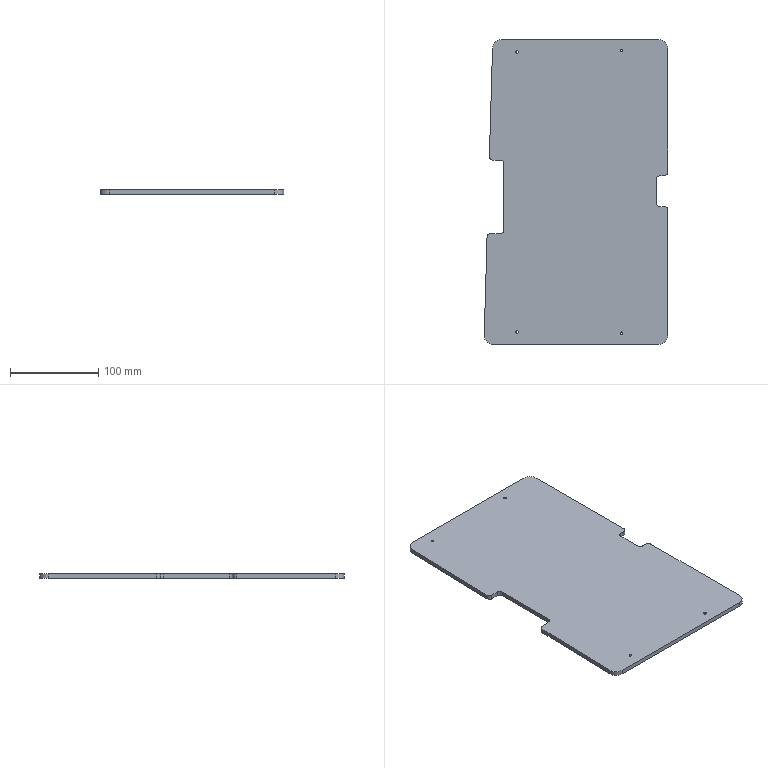Part | NX | features BREP 1 | 1 solid | 30 faces | box 207.864 x 345 x 5 mm | volume 340208 mm3 | cylinder 16 | plane 14 | commonest cylinder face diameters 8 x8 3 x4 20 x4
STEP:
#1=CARTESIAN_POINT('',(52.5,-322.5,0.));
#2=VERTEX_POINT('',#1);
#3=CARTESIAN_POINT('',(52.5,-180.495,0.));
#4=VERTEX_POINT('',#3);
#5=CARTESIAN_POINT('',(52.5,-332.5,0.));
#6=DIRECTION('',(0.,1.,0.));
#7=VECTOR('',#6,1000.);
#8=LINE('',#5,#7);
#9=EDGE_CURVE('',#2,#4,#8,.T.);
#10=ORIENTED_EDGE('',*,*,#9,.T.);
#11=CARTESIAN_POINT('',(52.5,-180.495,5.));
#12=VERTEX_POINT('',#11);
#13=CARTESIAN_POINT('',(52.5,-180.495,5.));
#14=DIRECTION('',(0.,0.,1.));
#15=VECTOR('',#14,1000.);
#16=LINE('',#13,#15);
#17=EDGE_CURVE('',#4,#12,#16,.T.);
#18=ORIENTED_EDGE('',*,*,#17,.T.);
#19=CARTESIAN_POINT('',(52.5,-322.5,5.));
#20=VERTEX_POINT('',#19);
#21=CARTESIAN_POINT('',(52.5,-332.5,5.));
#22=DIRECTION('',(0.,1.,0.));
#23=VECTOR('',#22,1000.);
#24=LINE('',#21,#23);
#25=EDGE_CURVE('',#20,#12,#24,.T.);
#26=ORIENTED_EDGE('',*,*,#25,.F.);
#27=CARTESIAN_POINT('',(52.5,-322.5,5.));
#28=DIRECTION('',(0.,0.,-1.));
#29=VECTOR('',#28,1000.);
#30=LINE('',#27,#29);
#31=EDGE_CURVE('',#20,#2,#30,.T.);
#32=ORIENTED_EDGE('',*,*,#31,.T.);
#33=EDGE_LOOP('',(#10,#18,#26,#32));
#34=FACE_BOUND('',#33,.T.);
#35=CARTESIAN_POINT('',(52.5,-332.5,5.));
#36=DIRECTION('',(-1.,0.,0.));
#37=DIRECTION('',(0.,1.,0.));
#38=AXIS2_PLACEMENT_3D('',#35,#36,#37);
#39=PLANE('',#38);
#40=ADVANCED_FACE('',(#34),#39,.F.);
#41=CARTESIAN_POINT('',(-152.133,-210.884,5.));
#42=VERTEX_POINT('',#41);
#43=CARTESIAN_POINT('',(-155.36,-322.21,5.));
#44=VERTEX_POINT('',#43);
#45=CARTESIAN_POINT('',(-145.658,12.5,5.));
#46=DIRECTION('',(-0.02897,-0.9996,0.));
#47=VECTOR('',#46,1000.);
#48=LINE('',#45,#47);
#49=EDGE_CURVE('',#42,#44,#48,.T.);
#50=ORIENTED_EDGE('',*,*,#49,.F.);
#51=CARTESIAN_POINT('',(-152.133,-210.884,0.));
#52=VERTEX_POINT('',#51);
#53=CARTESIAN_POINT('',(-152.133,-210.884,0.));
#54=DIRECTION('',(0.,0.,-1.));
#55=VECTOR('',#54,1000.);
#56=LINE('',#53,#55);
#57=EDGE_CURVE('',#42,#52,#56,.T.);
#58=ORIENTED_EDGE('',*,*,#57,.T.);
#59=CARTESIAN_POINT('',(-155.36,-322.21,0.));
#60=VERTEX_POINT('',#59);
#61=CARTESIAN_POINT('',(-145.658,12.5,0.));
#62=DIRECTION('',(-0.02897,-0.9996,0.));
#63=VECTOR('',#62,1000.);
#64=LINE('',#61,#63);
#65=EDGE_CURVE('',#52,#60,#64,.T.);
#66=ORIENTED_EDGE('',*,*,#65,.T.);
#67=CARTESIAN_POINT('',(-155.36,-322.21,5.));
#68=DIRECTION('',(0.,0.,1.));
#69=VECTOR('',#68,1000.);
#70=LINE('',#67,#69);
#71=EDGE_CURVE('',#60,#44,#70,.T.);
#72=ORIENTED_EDGE('',*,*,#71,.T.);
#73=EDGE_LOOP('',(#50,#58,#66,#72));
#74=FACE_BOUND('',#73,.T.);
#75=CARTESIAN_POINT('',(-145.658,12.5,5.));
#76=DIRECTION('',(0.9996,-0.02897,0.));
#77=DIRECTION('',(-0.02897,-0.9996,0.));
#78=AXIS2_PLACEMENT_3D('',#75,#76,#77);
#79=PLANE('',#78);
#80=ADVANCED_FACE('',(#74),#79,.F.);
#81=CARTESIAN_POINT('',(-145.94,2.79,0.));
#82=VERTEX_POINT('',#81);
#83=CARTESIAN_POINT('',(-149.495,-119.884,0.));
#84=VERTEX_POINT('',#83);
#85=CARTESIAN_POINT('',(-145.658,12.5,0.));
#86=DIRECTION('',(-0.02897,-0.9996,0.));
#87=VECTOR('',#86,1000.);
#88=LINE('',#85,#87);
#89=EDGE_CURVE('',#82,#84,#88,.T.);
#90=ORIENTED_EDGE('',*,*,#89,.T.);
#91=CARTESIAN_POINT('',(-149.495,-119.884,5.));
#92=VERTEX_POINT('',#91);
#93=CARTESIAN_POINT('',(-149.495,-119.884,5.));
#94=DIRECTION('',(0.,0.,1.));
#95=VECTOR('',#94,1000.);
#96=LINE('',#93,#95);
#97=EDGE_CURVE('',#84,#92,#96,.T.);
#98=ORIENTED_EDGE('',*,*,#97,.T.);
#99=CARTESIAN_POINT('',(-145.94,2.79,5.));
#100=VERTEX_POINT('',#99);
#101=CARTESIAN_POINT('',(-145.658,12.5,5.));
#102=DIRECTION('',(-0.02897,-0.9996,0.));
#103=VECTOR('',#102,1000.);
#104=LINE('',#101,#103);
#105=EDGE_CURVE('',#100,#92,#104,.T.);
#106=ORIENTED_EDGE('',*,*,#105,.F.);
#107=CARTESIAN_POINT('',(-145.94,2.79,5.));
#108=DIRECTION('',(0.,0.,-1.));
#109=VECTOR('',#108,1000.);
#110=LINE('',#107,#109);
#111=EDGE_CURVE('',#100,#82,#110,.T.);
#112=ORIENTED_EDGE('',*,*,#111,.T.);
#113=EDGE_LOOP('',(#90,#98,#106,#112));
#114=FACE_BOUND('',#113,.T.);
#115=CARTESIAN_POINT('',(-145.658,12.5,5.));
#116=DIRECTION('',(0.9996,-0.02897,0.));
#117=DIRECTION('',(-0.02897,-0.9996,0.));
#118=AXIS2_PLACEMENT_3D('',#115,#116,#117);
#119=PLANE('',#118);
#120=ADVANCED_FACE('',(#114),#119,.F.);
#121=CARTESIAN_POINT('',(0.,-318.5,5.));
#122=VERTEX_POINT('',#121);
#123=CARTESIAN_POINT('',(0.,-320.,5.));
#124=DIRECTION('',(0.,0.,-1.));
#125=DIRECTION('',(0.,1.,0.));
#126=AXIS2_PLACEMENT_3D('',#123,#124,#125);
#127=CIRCLE('',#126,1.5);
#128=EDGE_CURVE('',#122,#122,#127,.T.);
#129=ORIENTED_EDGE('',*,*,#128,.T.);
#130=EDGE_LOOP('',(#129));
#131=FACE_BOUND('',#130,.T.);
#132=CARTESIAN_POINT('',(-117.958,-3.,5.));
#133=VERTEX_POINT('',#132);
#134=CARTESIAN_POINT('',(-117.958,-1.5,5.));
#135=DIRECTION('',(0.,0.,1.));
#136=DIRECTION('',(0.,-1.,0.));
#137=AXIS2_PLACEMENT_3D('',#134,#135,#136);
#138=CIRCLE('',#137,1.5);
#139=EDGE_CURVE('',#133,#133,#138,.T.);
#140=ORIENTED_EDGE('',*,*,#139,.F.);
#141=EDGE_LOOP('',(#140));
#142=FACE_BOUND('',#141,.T.);
#143=CARTESIAN_POINT('',(-117.958,-317.,5.));
#144=VERTEX_POINT('',#143);
#145=CARTESIAN_POINT('',(-117.958,-318.5,5.));
#146=DIRECTION('',(0.,0.,-1.));
#147=DIRECTION('',(0.,1.,0.));
#148=AXIS2_PLACEMENT_3D('',#145,#146,#147);
#149=CIRCLE('',#148,1.5);
#150=EDGE_CURVE('',#144,#144,#149,.T.);
#151=ORIENTED_EDGE('',*,*,#150,.T.);
#152=EDGE_LOOP('',(#151));
#153=FACE_BOUND('',#152,.T.);
#154=CARTESIAN_POINT('',(0.,-1.5,5.));
#155=VERTEX_POINT('',#154);
#156=CARTESIAN_POINT('',(0.,0.,5.));
#157=DIRECTION('',(0.,0.,1.));
#158=DIRECTION('',(0.,-1.,0.));
#159=AXIS2_PLACEMENT_3D('',#156,#157,#158);
#160=CIRCLE('',#159,1.5);
#161=EDGE_CURVE('',#155,#155,#160,.T.);
#162=ORIENTED_EDGE('',*,*,#161,.F.);
#163=EDGE_LOOP('',(#162));
#164=FACE_BOUND('',#163,.T.);
#165=CARTESIAN_POINT('',(-148.135,-207.,5.));
#166=VERTEX_POINT('',#165);
#167=CARTESIAN_POINT('',(-137.,-207.,5.));
#168=VERTEX_POINT('',#167);
#169=CARTESIAN_POINT('',(0.,-207.,5.));
#170=DIRECTION('',(1.,0.,0.));
#171=VECTOR('',#170,1000.);
#172=LINE('',#169,#171);
#173=EDGE_CURVE('',#166,#168,#172,.T.);
#174=ORIENTED_EDGE('',*,*,#173,.F.);
#175=CARTESIAN_POINT('',(-148.135,-211.,5.));
#176=DIRECTION('',(0.,0.,1.));
#177=DIRECTION('',(-1.,0.,0.));
#178=AXIS2_PLACEMENT_3D('',#175,#176,#177);
#179=CIRCLE('',#178,4.);
#180=EDGE_CURVE('',#166,#42,#179,.T.);
#181=ORIENTED_EDGE('',*,*,#180,.T.);
#182=ORIENTED_EDGE('',*,*,#49,.T.);
#183=CARTESIAN_POINT('',(-145.364,-332.5,5.));
#184=VERTEX_POINT('',#183);
#185=CARTESIAN_POINT('',(-145.364,-322.5,5.));
#186=DIRECTION('',(0.,0.,1.));
#187=DIRECTION('',(-1.,0.,0.));
#188=AXIS2_PLACEMENT_3D('',#185,#186,#187);
#189=CIRCLE('',#188,10.);
#190=EDGE_CURVE('',#44,#184,#189,.T.);
#191=ORIENTED_EDGE('',*,*,#190,.T.);
#192=CARTESIAN_POINT('',(42.5,-332.5,5.));
#193=VERTEX_POINT('',#192);
#194=CARTESIAN_POINT('',(-155.658,-332.5,5.));
#195=DIRECTION('',(1.,0.,0.));
#196=VECTOR('',#195,1000.);
#197=LINE('',#194,#196);
#198=EDGE_CURVE('',#184,#193,#197,.T.);
#199=ORIENTED_EDGE('',*,*,#198,.T.);
#200=CARTESIAN_POINT('',(42.5,-322.5,5.));
#201=DIRECTION('',(0.,0.,1.));
#202=DIRECTION('',(-1.,0.,0.));
#203=AXIS2_PLACEMENT_3D('',#200,#201,#202);
#204=CIRCLE('',#203,10.);
#205=EDGE_CURVE('',#193,#20,#204,.T.);
#206=ORIENTED_EDGE('',*,*,#205,.T.);
#207=ORIENTED_EDGE('',*,*,#25,.T.);
#208=CARTESIAN_POINT('',(48.5,-176.495,5.));
#209=VERTEX_POINT('',#208);
#210=CARTESIAN_POINT('',(48.5,-180.495,5.));
#211=DIRECTION('',(0.,0.,1.));
#212=DIRECTION('',(-1.,0.,0.));
#213=AXIS2_PLACEMENT_3D('',#210,#211,#212);
#214=CIRCLE('',#213,4.);
#215=EDGE_CURVE('',#12,#209,#214,.T.);
#216=ORIENTED_EDGE('',*,*,#215,.T.);
#217=CARTESIAN_POINT('',(43.5,-176.495,5.));
#218=VERTEX_POINT('',#217);
#219=CARTESIAN_POINT('',(0.,-176.495,5.));
#220=DIRECTION('',(1.,0.,0.));
#221=VECTOR('',#220,1000.);
#222=LINE('',#219,#221);
#223=EDGE_CURVE('',#218,#209,#222,.T.);
#224=ORIENTED_EDGE('',*,*,#223,.F.);
#225=CARTESIAN_POINT('',(39.5,-172.495,5.));
#226=VERTEX_POINT('',#225);
#227=CARTESIAN_POINT('',(43.5,-172.495,5.));
#228=DIRECTION('',(0.,0.,-1.));
#229=DIRECTION('',(-1.,0.,0.));
#230=AXIS2_PLACEMENT_3D('',#227,#228,#229);
#231=CIRCLE('',#230,4.);
#232=EDGE_CURVE('',#218,#226,#231,.T.);
#233=ORIENTED_EDGE('',*,*,#232,.T.);
#234=CARTESIAN_POINT('',(39.5,-145.495,5.));
#235=VERTEX_POINT('',#234);
#236=CARTESIAN_POINT('',(39.5,-320.,5.));
#237=DIRECTION('',(0.,-1.,0.));
#238=VECTOR('',#237,1000.);
#239=LINE('',#236,#238);
#240=EDGE_CURVE('',#235,#226,#239,.T.);
#241=ORIENTED_EDGE('',*,*,#240,.F.);
#242=CARTESIAN_POINT('',(43.5,-141.495,5.));
#243=VERTEX_POINT('',#242);
#244=CARTESIAN_POINT('',(43.5,-145.495,5.));
#245=DIRECTION('',(0.,0.,-1.));
#246=DIRECTION('',(-1.,0.,0.));
#247=AXIS2_PLACEMENT_3D('',#244,#245,#246);
#248=CIRCLE('',#247,4.);
#249=EDGE_CURVE('',#235,#243,#248,.T.);
#250=ORIENTED_EDGE('',*,*,#249,.T.);
#251=CARTESIAN_POINT('',(48.5,-141.495,5.));
#252=VERTEX_POINT('',#251);
#253=CARTESIAN_POINT('',(0.,-141.495,5.));
#254=DIRECTION('',(-1.,0.,0.));
#255=VECTOR('',#254,1000.);
#256=LINE('',#253,#255);
#257=EDGE_CURVE('',#252,#243,#256,.T.);
#258=ORIENTED_EDGE('',*,*,#257,.F.);
#259=CARTESIAN_POINT('',(52.5,-137.495,5.));
#260=VERTEX_POINT('',#259);
#261=CARTESIAN_POINT('',(48.5,-137.495,5.));
#262=DIRECTION('',(0.,0.,1.));
#263=DIRECTION('',(-1.,0.,0.));
#264=AXIS2_PLACEMENT_3D('',#261,#262,#263);
#265=CIRCLE('',#264,4.);
#266=EDGE_CURVE('',#252,#260,#265,.T.);
#267=ORIENTED_EDGE('',*,*,#266,.T.);
#268=CARTESIAN_POINT('',(52.5,2.5,5.));
#269=VERTEX_POINT('',#268);
#270=CARTESIAN_POINT('',(52.5,-332.5,5.));
#271=DIRECTION('',(0.,1.,0.));
#272=VECTOR('',#271,1000.);
#273=LINE('',#270,#272);
#274=EDGE_CURVE('',#260,#269,#273,.T.);
#275=ORIENTED_EDGE('',*,*,#274,.T.);
#276=CARTESIAN_POINT('',(42.5,12.5,5.));
#277=VERTEX_POINT('',#276);
#278=CARTESIAN_POINT('',(42.5,2.5,5.));
#279=DIRECTION('',(0.,0.,1.));
#280=DIRECTION('',(-1.,0.,0.));
#281=AXIS2_PLACEMENT_3D('',#278,#279,#280);
#282=CIRCLE('',#281,10.);
#283=EDGE_CURVE('',#269,#277,#282,.T.);
#284=ORIENTED_EDGE('',*,*,#283,.T.);
#285=CARTESIAN_POINT('',(-135.944,12.5,5.));
#286=VERTEX_POINT('',#285);
#287=CARTESIAN_POINT('',(52.5,12.5,5.));
#288=DIRECTION('',(-1.,0.,0.));
#289=VECTOR('',#288,1000.);
#290=LINE('',#287,#289);
#291=EDGE_CURVE('',#277,#286,#290,.T.);
#292=ORIENTED_EDGE('',*,*,#291,.T.);
#293=CARTESIAN_POINT('',(-135.944,2.5,5.));
#294=DIRECTION('',(0.,0.,1.));
#295=DIRECTION('',(-1.,0.,0.));
#296=AXIS2_PLACEMENT_3D('',#293,#294,#295);
#297=CIRCLE('',#296,10.);
#298=EDGE_CURVE('',#286,#100,#297,.T.);
#299=ORIENTED_EDGE('',*,*,#298,.T.);
#300=ORIENTED_EDGE('',*,*,#105,.T.);
#301=CARTESIAN_POINT('',(-145.497,-124.,5.));
#302=VERTEX_POINT('',#301);
#303=CARTESIAN_POINT('',(-145.497,-120.,5.));
#304=DIRECTION('',(0.,0.,1.));
#305=DIRECTION('',(-1.,0.,0.));
#306=AXIS2_PLACEMENT_3D('',#303,#304,#305);
#307=CIRCLE('',#306,4.);
#308=EDGE_CURVE('',#92,#302,#307,.T.);
#309=ORIENTED_EDGE('',*,*,#308,.T.);
#310=CARTESIAN_POINT('',(-137.,-124.,5.));
#311=VERTEX_POINT('',#310);
#312=CARTESIAN_POINT('',(0.,-124.,5.));
#313=DIRECTION('',(-1.,0.,0.));
#314=VECTOR('',#313,1000.);
#315=LINE('',#312,#314);
#316=EDGE_CURVE('',#311,#302,#315,.T.);
#317=ORIENTED_EDGE('',*,*,#316,.F.);
#318=CARTESIAN_POINT('',(-133.,-128.,5.));
#319=VERTEX_POINT('',#318);
#320=CARTESIAN_POINT('',(-137.,-128.,5.));
#321=DIRECTION('',(0.,0.,-1.));
#322=DIRECTION('',(-1.,0.,0.));
#323=AXIS2_PLACEMENT_3D('',#320,#321,#322);
#324=CIRCLE('',#323,4.);
#325=EDGE_CURVE('',#311,#319,#324,.T.);
#326=ORIENTED_EDGE('',*,*,#325,.T.);
#327=CARTESIAN_POINT('',(-133.,-203.,5.));
#328=VERTEX_POINT('',#327);
#329=CARTESIAN_POINT('',(-133.,-320.,5.));
#330=DIRECTION('',(0.,1.,0.));
#331=VECTOR('',#330,1000.);
#332=LINE('',#329,#331);
#333=EDGE_CURVE('',#328,#319,#332,.T.);
#334=ORIENTED_EDGE('',*,*,#333,.F.);
#335=CARTESIAN_POINT('',(-137.,-203.,5.));
#336=DIRECTION('',(0.,0.,-1.));
#337=DIRECTION('',(-1.,0.,0.));
#338=AXIS2_PLACEMENT_3D('',#335,#336,#337);
#339=CIRCLE('',#338,4.);
#340=EDGE_CURVE('',#328,#168,#339,.T.);
#341=ORIENTED_EDGE('',*,*,#340,.T.);
#342=EDGE_LOOP('',(#174,#181,#182,#191,#199,#206,#207,#216,#224,#233,#241,#250,#258,#267,#275,#284,#292,#299,#300,#309,#317,#326,#334,#341));
#343=FACE_BOUND('',#342,.T.);
#344=CARTESIAN_POINT('',(0.,-320.,5.));
#345=DIRECTION('',(0.,0.,-1.));
#346=DIRECTION('',(1.,0.,0.));
#347=AXIS2_PLACEMENT_3D('',#344,#345,#346);
#348=PLANE('',#347);
#349=ADVANCED_FACE('',(#131,#142,#153,#164,#343),#348,.F.);
#350=CARTESIAN_POINT('',(0.,-318.5,0.));
#351=VERTEX_POINT('',#350);
#352=CARTESIAN_POINT('',(0.,-320.,0.));
#353=DIRECTION('',(0.,0.,-1.));
#354=DIRECTION('',(0.,1.,0.));
#355=AXIS2_PLACEMENT_3D('',#352,#353,#354);
#356=CIRCLE('',#355,1.5);
#357=EDGE_CURVE('',#351,#351,#356,.T.);
#358=ORIENTED_EDGE('',*,*,#357,.F.);
#359=EDGE_LOOP('',(#358));
#360=FACE_BOUND('',#359,.T.);
#361=CARTESIAN_POINT('',(-117.958,-3.,0.));
#362=VERTEX_POINT('',#361);
#363=CARTESIAN_POINT('',(-117.958,-1.5,0.));
#364=DIRECTION('',(0.,0.,1.));
#365=DIRECTION('',(0.,-1.,0.));
#366=AXIS2_PLACEMENT_3D('',#363,#364,#365);
#367=CIRCLE('',#366,1.5);
#368=EDGE_CURVE('',#362,#362,#367,.T.);
#369=ORIENTED_EDGE('',*,*,#368,.T.);
#370=EDGE_LOOP('',(#369));
#371=FACE_BOUND('',#370,.T.);
#372=CARTESIAN_POINT('',(-117.958,-317.,0.));
#373=VERTEX_POINT('',#372);
#374=CARTESIAN_POINT('',(-117.958,-318.5,0.));
#375=DIRECTION('',(0.,0.,-1.));
#376=DIRECTION('',(0.,1.,0.));
#377=AXIS2_PLACEMENT_3D('',#374,#375,#376);
#378=CIRCLE('',#377,1.5);
#379=EDGE_CURVE('',#373,#373,#378,.T.);
#380=ORIENTED_EDGE('',*,*,#379,.F.);
#381=EDGE_LOOP('',(#380));
#382=FACE_BOUND('',#381,.T.);
#383=CARTESIAN_POINT('',(0.,-1.5,0.));
#384=VERTEX_POINT('',#383);
#385=CARTESIAN_POINT('',(0.,0.,0.));
#386=DIRECTION('',(0.,0.,1.));
#387=DIRECTION('',(0.,-1.,0.));
#388=AXIS2_PLACEMENT_3D('',#385,#386,#387);
#389=CIRCLE('',#388,1.5);
#390=EDGE_CURVE('',#384,#384,#389,.T.);
#391=ORIENTED_EDGE('',*,*,#390,.T.);
#392=EDGE_LOOP('',(#391));
#393=FACE_BOUND('',#392,.T.);
#394=ORIENTED_EDGE('',*,*,#65,.F.);
#395=CARTESIAN_POINT('',(-148.135,-207.,0.));
#396=VERTEX_POINT('',#395);
#397=CARTESIAN_POINT('',(-148.135,-211.,0.));
#398=DIRECTION('',(0.,0.,-1.));
#399=DIRECTION('',(-1.,0.,0.));
#400=AXIS2_PLACEMENT_3D('',#397,#398,#399);
#401=CIRCLE('',#400,4.);
#402=EDGE_CURVE('',#52,#396,#401,.T.);
#403=ORIENTED_EDGE('',*,*,#402,.T.);
#404=CARTESIAN_POINT('',(-137.,-207.,0.));
#405=VERTEX_POINT('',#404);
#406=CARTESIAN_POINT('',(0.,-207.,0.));
#407=DIRECTION('',(1.,0.,0.));
#408=VECTOR('',#407,1000.);
#409=LINE('',#406,#408);
#410=EDGE_CURVE('',#396,#405,#409,.T.);
#411=ORIENTED_EDGE('',*,*,#410,.T.);
#412=CARTESIAN_POINT('',(-133.,-203.,0.));
#413=VERTEX_POINT('',#412);
#414=CARTESIAN_POINT('',(-137.,-203.,0.));
#415=DIRECTION('',(0.,0.,1.));
#416=DIRECTION('',(-1.,0.,0.));
#417=AXIS2_PLACEMENT_3D('',#414,#415,#416);
#418=CIRCLE('',#417,4.);
#419=EDGE_CURVE('',#405,#413,#418,.T.);
#420=ORIENTED_EDGE('',*,*,#419,.T.);
#421=CARTESIAN_POINT('',(-133.,-128.,0.));
#422=VERTEX_POINT('',#421);
#423=CARTESIAN_POINT('',(-133.,-320.,0.));
#424=DIRECTION('',(0.,1.,0.));
#425=VECTOR('',#424,1000.);
#426=LINE('',#423,#425);
#427=EDGE_CURVE('',#413,#422,#426,.T.);
#428=ORIENTED_EDGE('',*,*,#427,.T.);
#429=CARTESIAN_POINT('',(-137.,-124.,0.));
#430=VERTEX_POINT('',#429);
#431=CARTESIAN_POINT('',(-137.,-128.,0.));
#432=DIRECTION('',(0.,0.,1.));
#433=DIRECTION('',(-1.,0.,0.));
#434=AXIS2_PLACEMENT_3D('',#431,#432,#433);
#435=CIRCLE('',#434,4.);
#436=EDGE_CURVE('',#422,#430,#435,.T.);
#437=ORIENTED_EDGE('',*,*,#436,.T.);
#438=CARTESIAN_POINT('',(-145.497,-124.,0.));
#439=VERTEX_POINT('',#438);
#440=CARTESIAN_POINT('',(0.,-124.,0.));
#441=DIRECTION('',(-1.,0.,0.));
#442=VECTOR('',#441,1000.);
#443=LINE('',#440,#442);
#444=EDGE_CURVE('',#430,#439,#443,.T.);
#445=ORIENTED_EDGE('',*,*,#444,.T.);
#446=CARTESIAN_POINT('',(-145.497,-120.,0.));
#447=DIRECTION('',(0.,0.,-1.));
#448=DIRECTION('',(-1.,0.,0.));
#449=AXIS2_PLACEMENT_3D('',#446,#447,#448);
#450=CIRCLE('',#449,4.);
#451=EDGE_CURVE('',#439,#84,#450,.T.);
#452=ORIENTED_EDGE('',*,*,#451,.T.);
#453=ORIENTED_EDGE('',*,*,#89,.F.);
#454=CARTESIAN_POINT('',(-135.944,12.5,0.));
#455=VERTEX_POINT('',#454);
#456=CARTESIAN_POINT('',(-135.944,2.5,0.));
#457=DIRECTION('',(0.,0.,-1.));
#458=DIRECTION('',(-1.,0.,0.));
#459=AXIS2_PLACEMENT_3D('',#456,#457,#458);
#460=CIRCLE('',#459,10.);
#461=EDGE_CURVE('',#82,#455,#460,.T.);
#462=ORIENTED_EDGE('',*,*,#461,.T.);
#463=CARTESIAN_POINT('',(42.5,12.5,0.));
#464=VERTEX_POINT('',#463);
#465=CARTESIAN_POINT('',(52.5,12.5,0.));
#466=DIRECTION('',(-1.,0.,0.));
#467=VECTOR('',#466,1000.);
#468=LINE('',#465,#467);
#469=EDGE_CURVE('',#464,#455,#468,.T.);
#470=ORIENTED_EDGE('',*,*,#469,.F.);
#471=CARTESIAN_POINT('',(52.5,2.5,0.));
#472=VERTEX_POINT('',#471);
#473=CARTESIAN_POINT('',(42.5,2.5,0.));
#474=DIRECTION('',(0.,0.,-1.));
#475=DIRECTION('',(-1.,0.,0.));
#476=AXIS2_PLACEMENT_3D('',#473,#474,#475);
#477=CIRCLE('',#476,10.);
#478=EDGE_CURVE('',#464,#472,#477,.T.);
#479=ORIENTED_EDGE('',*,*,#478,.T.);
#480=CARTESIAN_POINT('',(52.5,-137.495,0.));
#481=VERTEX_POINT('',#480);
#482=CARTESIAN_POINT('',(52.5,-332.5,0.));
#483=DIRECTION('',(0.,1.,0.));
#484=VECTOR('',#483,1000.);
#485=LINE('',#482,#484);
#486=EDGE_CURVE('',#481,#472,#485,.T.);
#487=ORIENTED_EDGE('',*,*,#486,.F.);
#488=CARTESIAN_POINT('',(48.5,-141.495,0.));
#489=VERTEX_POINT('',#488);
#490=CARTESIAN_POINT('',(48.5,-137.495,0.));
#491=DIRECTION('',(0.,0.,-1.));
#492=DIRECTION('',(-1.,0.,0.));
#493=AXIS2_PLACEMENT_3D('',#490,#491,#492);
#494=CIRCLE('',#493,4.);
#495=EDGE_CURVE('',#481,#489,#494,.T.);
#496=ORIENTED_EDGE('',*,*,#495,.T.);
#497=CARTESIAN_POINT('',(43.5,-141.495,0.));
#498=VERTEX_POINT('',#497);
#499=CARTESIAN_POINT('',(0.,-141.495,0.));
#500=DIRECTION('',(-1.,0.,0.));
#501=VECTOR('',#500,1000.);
#502=LINE('',#499,#501);
#503=EDGE_CURVE('',#489,#498,#502,.T.);
#504=ORIENTED_EDGE('',*,*,#503,.T.);
#505=CARTESIAN_POINT('',(39.5,-145.495,0.));
#506=VERTEX_POINT('',#505);
#507=CARTESIAN_POINT('',(43.5,-145.495,0.));
#508=DIRECTION('',(0.,0.,1.));
#509=DIRECTION('',(-1.,0.,0.));
#510=AXIS2_PLACEMENT_3D('',#507,#508,#509);
#511=CIRCLE('',#510,4.);
#512=EDGE_CURVE('',#498,#506,#511,.T.);
#513=ORIENTED_EDGE('',*,*,#512,.T.);
#514=CARTESIAN_POINT('',(39.5,-172.495,0.));
#515=VERTEX_POINT('',#514);
#516=CARTESIAN_POINT('',(39.5,-320.,0.));
#517=DIRECTION('',(0.,-1.,0.));
#518=VECTOR('',#517,1000.);
#519=LINE('',#516,#518);
#520=EDGE_CURVE('',#506,#515,#519,.T.);
#521=ORIENTED_EDGE('',*,*,#520,.T.);
#522=CARTESIAN_POINT('',(43.5,-176.495,0.));
#523=VERTEX_POINT('',#522);
#524=CARTESIAN_POINT('',(43.5,-172.495,0.));
#525=DIRECTION('',(0.,0.,1.));
#526=DIRECTION('',(-1.,0.,0.));
#527=AXIS2_PLACEMENT_3D('',#524,#525,#526);
#528=CIRCLE('',#527,4.);
#529=EDGE_CURVE('',#515,#523,#528,.T.);
#530=ORIENTED_EDGE('',*,*,#529,.T.);
#531=CARTESIAN_POINT('',(48.5,-176.495,0.));
#532=VERTEX_POINT('',#531);
#533=CARTESIAN_POINT('',(0.,-176.495,0.));
#534=DIRECTION('',(1.,0.,0.));
#535=VECTOR('',#534,1000.);
#536=LINE('',#533,#535);
#537=EDGE_CURVE('',#523,#532,#536,.T.);
#538=ORIENTED_EDGE('',*,*,#537,.T.);
#539=CARTESIAN_POINT('',(48.5,-180.495,0.));
#540=DIRECTION('',(0.,0.,-1.));
#541=DIRECTION('',(-1.,0.,0.));
#542=AXIS2_PLACEMENT_3D('',#539,#540,#541);
#543=CIRCLE('',#542,4.);
#544=EDGE_CURVE('',#532,#4,#543,.T.);
#545=ORIENTED_EDGE('',*,*,#544,.T.);
#546=ORIENTED_EDGE('',*,*,#9,.F.);
#547=CARTESIAN_POINT('',(42.5,-332.5,0.));
#548=VERTEX_POINT('',#547);
#549=CARTESIAN_POINT('',(42.5,-322.5,0.));
#550=DIRECTION('',(0.,0.,-1.));
#551=DIRECTION('',(-1.,0.,0.));
#552=AXIS2_PLACEMENT_3D('',#549,#550,#551);
#553=CIRCLE('',#552,10.);
#554=EDGE_CURVE('',#2,#548,#553,.T.);
#555=ORIENTED_EDGE('',*,*,#554,.T.);
#556=CARTESIAN_POINT('',(-145.364,-332.5,0.));
#557=VERTEX_POINT('',#556);
#558=CARTESIAN_POINT('',(-155.658,-332.5,0.));
#559=DIRECTION('',(1.,0.,0.));
#560=VECTOR('',#559,1000.);
#561=LINE('',#558,#560);
#562=EDGE_CURVE('',#557,#548,#561,.T.);
#563=ORIENTED_EDGE('',*,*,#562,.F.);
#564=CARTESIAN_POINT('',(-145.364,-322.5,0.));
#565=DIRECTION('',(0.,0.,-1.));
#566=DIRECTION('',(-1.,0.,0.));
#567=AXIS2_PLACEMENT_3D('',#564,#565,#566);
#568=CIRCLE('',#567,10.);
#569=EDGE_CURVE('',#557,#60,#568,.T.);
#570=ORIENTED_EDGE('',*,*,#569,.T.);
#571=EDGE_LOOP('',(#394,#403,#411,#420,#428,#437,#445,#452,#453,#462,#470,#479,#487,#496,#504,#513,#521,#530,#538,#545,#546,#555,#563,#570));
#572=FACE_BOUND('',#571,.T.);
#573=CARTESIAN_POINT('',(0.,-320.,0.));
#574=DIRECTION('',(0.,0.,-1.));
#575=DIRECTION('',(1.,0.,0.));
#576=AXIS2_PLACEMENT_3D('',#573,#574,#575);
#577=PLANE('',#576);
#578=ADVANCED_FACE('',(#360,#371,#382,#393,#572),#577,.T.);
#579=ORIENTED_EDGE('',*,*,#198,.F.);
#580=CARTESIAN_POINT('',(-145.364,-332.5,5.));
#581=DIRECTION('',(0.,0.,-1.));
#582=VECTOR('',#581,1000.);
#583=LINE('',#580,#582);
#584=EDGE_CURVE('',#184,#557,#583,.T.);
#585=ORIENTED_EDGE('',*,*,#584,.T.);
#586=ORIENTED_EDGE('',*,*,#562,.T.);
#587=CARTESIAN_POINT('',(42.5,-332.5,5.));
#588=DIRECTION('',(0.,0.,1.));
#589=VECTOR('',#588,1000.);
#590=LINE('',#587,#589);
#591=EDGE_CURVE('',#548,#193,#590,.T.);
#592=ORIENTED_EDGE('',*,*,#591,.T.);
#593=EDGE_LOOP('',(#579,#585,#586,#592));
#594=FACE_BOUND('',#593,.T.);
#595=CARTESIAN_POINT('',(-155.658,-332.5,5.));
#596=DIRECTION('',(0.,1.,0.));
#597=DIRECTION('',(1.,0.,0.));
#598=AXIS2_PLACEMENT_3D('',#595,#596,#597);
#599=PLANE('',#598);
#600=ADVANCED_FACE('',(#594),#599,.F.);
#601=ORIENTED_EDGE('',*,*,#274,.F.);
#602=CARTESIAN_POINT('',(52.5,-137.495,0.));
#603=DIRECTION('',(0.,0.,-1.));
#604=VECTOR('',#603,1000.);
#605=LINE('',#602,#604);
#606=EDGE_CURVE('',#260,#481,#605,.T.);
#607=ORIENTED_EDGE('',*,*,#606,.T.);
#608=ORIENTED_EDGE('',*,*,#486,.T.);
#609=CARTESIAN_POINT('',(52.5,2.5,5.));
#610=DIRECTION('',(0.,0.,1.));
#611=VECTOR('',#610,1000.);
#612=LINE('',#609,#611);
#613=EDGE_CURVE('',#472,#269,#612,.T.);
#614=ORIENTED_EDGE('',*,*,#613,.T.);
#615=EDGE_LOOP('',(#601,#607,#608,#614));
#616=FACE_BOUND('',#615,.T.);
#617=CARTESIAN_POINT('',(52.5,-332.5,5.));
#618=DIRECTION('',(-1.,0.,0.));
#619=DIRECTION('',(0.,1.,0.));
#620=AXIS2_PLACEMENT_3D('',#617,#618,#619);
#621=PLANE('',#620);
#622=ADVANCED_FACE('',(#616),#621,.F.);
#623=ORIENTED_EDGE('',*,*,#150,.F.);
#624=EDGE_LOOP('',(#623));
#625=FACE_BOUND('',#624,.T.);
#626=ORIENTED_EDGE('',*,*,#379,.T.);
#627=EDGE_LOOP('',(#626));
#628=FACE_BOUND('',#627,.T.);
#629=CARTESIAN_POINT('',(-117.958,-318.5,5.));
#630=DIRECTION('',(0.,0.,-1.));
#631=DIRECTION('',(1.,0.,0.));
#632=AXIS2_PLACEMENT_3D('',#629,#630,#631);
#633=CYLINDRICAL_SURFACE('',#632,1.5);
#634=ADVANCED_FACE('',(#625,#628),#633,.F.);
#635=ORIENTED_EDGE('',*,*,#139,.T.);
#636=EDGE_LOOP('',(#635));
#637=FACE_BOUND('',#636,.T.);
#638=ORIENTED_EDGE('',*,*,#368,.F.);
#639=EDGE_LOOP('',(#638));
#640=FACE_BOUND('',#639,.T.);
#641=CARTESIAN_POINT('',(-117.958,-1.5,5.));
#642=DIRECTION('',(0.,0.,-1.));
#643=DIRECTION('',(1.,0.,0.));
#644=AXIS2_PLACEMENT_3D('',#641,#642,#643);
#645=CYLINDRICAL_SURFACE('',#644,1.5);
#646=ADVANCED_FACE('',(#637,#640),#645,.F.);
#647=ORIENTED_EDGE('',*,*,#128,.F.);
#648=EDGE_LOOP('',(#647));
#649=FACE_BOUND('',#648,.T.);
#650=ORIENTED_EDGE('',*,*,#357,.T.);
#651=EDGE_LOOP('',(#650));
#652=FACE_BOUND('',#651,.T.);
#653=CARTESIAN_POINT('',(0.,-320.,5.));
#654=DIRECTION('',(0.,0.,-1.));
#655=DIRECTION('',(1.,0.,0.));
#656=AXIS2_PLACEMENT_3D('',#653,#654,#655);
#657=CYLINDRICAL_SURFACE('',#656,1.5);
#658=ADVANCED_FACE('',(#649,#652),#657,.F.);
#659=ORIENTED_EDGE('',*,*,#469,.T.);
#660=CARTESIAN_POINT('',(-135.944,12.5,5.));
#661=DIRECTION('',(0.,0.,1.));
#662=VECTOR('',#661,1000.);
#663=LINE('',#660,#662);
#664=EDGE_CURVE('',#455,#286,#663,.T.);
#665=ORIENTED_EDGE('',*,*,#664,.T.);
#666=ORIENTED_EDGE('',*,*,#291,.F.);
#667=CARTESIAN_POINT('',(42.5,12.5,5.));
#668=DIRECTION('',(0.,0.,-1.));
#669=VECTOR('',#668,1000.);
#670=LINE('',#667,#669);
#671=EDGE_CURVE('',#277,#464,#670,.T.);
#672=ORIENTED_EDGE('',*,*,#671,.T.);
#673=EDGE_LOOP('',(#659,#665,#666,#672));
#674=FACE_BOUND('',#673,.T.);
#675=CARTESIAN_POINT('',(52.5,12.5,5.));
#676=DIRECTION('',(0.,-1.,0.));
#677=DIRECTION('',(0.,0.,1.));
#678=AXIS2_PLACEMENT_3D('',#675,#676,#677);
#679=PLANE('',#678);
#680=ADVANCED_FACE('',(#674),#679,.F.);
#681=ORIENTED_EDGE('',*,*,#161,.T.);
#682=EDGE_LOOP('',(#681));
#683=FACE_BOUND('',#682,.T.);
#684=ORIENTED_EDGE('',*,*,#390,.F.);
#685=EDGE_LOOP('',(#684));
#686=FACE_BOUND('',#685,.T.);
#687=CARTESIAN_POINT('',(0.,0.,5.));
#688=DIRECTION('',(0.,0.,-1.));
#689=DIRECTION('',(1.,0.,0.));
#690=AXIS2_PLACEMENT_3D('',#687,#688,#689);
#691=CYLINDRICAL_SURFACE('',#690,1.5);
#692=ADVANCED_FACE('',(#683,#686),#691,.F.);
#693=ORIENTED_EDGE('',*,*,#190,.F.);
#694=ORIENTED_EDGE('',*,*,#71,.F.);
#695=ORIENTED_EDGE('',*,*,#569,.F.);
#696=ORIENTED_EDGE('',*,*,#584,.F.);
#697=EDGE_LOOP('',(#693,#694,#695,#696));
#698=FACE_BOUND('',#697,.T.);
#699=CARTESIAN_POINT('',(-145.364,-322.5,5.));
#700=DIRECTION('',(0.,0.,-1.));
#701=DIRECTION('',(1.,0.,0.));
#702=AXIS2_PLACEMENT_3D('',#699,#700,#701);
#703=CYLINDRICAL_SURFACE('',#702,10.);
#704=ADVANCED_FACE('',(#698),#703,.T.);
#705=ORIENTED_EDGE('',*,*,#298,.F.);
#706=ORIENTED_EDGE('',*,*,#664,.F.);
#707=ORIENTED_EDGE('',*,*,#461,.F.);
#708=ORIENTED_EDGE('',*,*,#111,.F.);
#709=EDGE_LOOP('',(#705,#706,#707,#708));
#710=FACE_BOUND('',#709,.T.);
#711=CARTESIAN_POINT('',(-135.944,2.5,5.));
#712=DIRECTION('',(0.,0.,-1.));
#713=DIRECTION('',(1.,0.,0.));
#714=AXIS2_PLACEMENT_3D('',#711,#712,#713);
#715=CYLINDRICAL_SURFACE('',#714,10.);
#716=ADVANCED_FACE('',(#710),#715,.T.);
#717=ORIENTED_EDGE('',*,*,#283,.F.);
#718=ORIENTED_EDGE('',*,*,#613,.F.);
#719=ORIENTED_EDGE('',*,*,#478,.F.);
#720=ORIENTED_EDGE('',*,*,#671,.F.);
#721=EDGE_LOOP('',(#717,#718,#719,#720));
#722=FACE_BOUND('',#721,.T.);
#723=CARTESIAN_POINT('',(42.5,2.5,5.));
#724=DIRECTION('',(0.,0.,-1.));
#725=DIRECTION('',(1.,0.,0.));
#726=AXIS2_PLACEMENT_3D('',#723,#724,#725);
#727=CYLINDRICAL_SURFACE('',#726,10.);
#728=ADVANCED_FACE('',(#722),#727,.T.);
#729=ORIENTED_EDGE('',*,*,#205,.F.);
#730=ORIENTED_EDGE('',*,*,#591,.F.);
#731=ORIENTED_EDGE('',*,*,#554,.F.);
#732=ORIENTED_EDGE('',*,*,#31,.F.);
#733=EDGE_LOOP('',(#729,#730,#731,#732));
#734=FACE_BOUND('',#733,.T.);
#735=CARTESIAN_POINT('',(42.5,-322.5,5.));
#736=DIRECTION('',(0.,0.,-1.));
#737=DIRECTION('',(1.,0.,0.));
#738=AXIS2_PLACEMENT_3D('',#735,#736,#737);
#739=CYLINDRICAL_SURFACE('',#738,10.);
#740=ADVANCED_FACE('',(#734),#739,.T.);
#741=ORIENTED_EDGE('',*,*,#410,.F.);
#742=CARTESIAN_POINT('',(-148.135,-207.,5.));
#743=DIRECTION('',(0.,0.,1.));
#744=VECTOR('',#743,1000.);
#745=LINE('',#742,#744);
#746=EDGE_CURVE('',#396,#166,#745,.T.);
#747=ORIENTED_EDGE('',*,*,#746,.T.);
#748=ORIENTED_EDGE('',*,*,#173,.T.);
#749=CARTESIAN_POINT('',(-137.,-207.,0.));
#750=DIRECTION('',(0.,0.,-1.));
#751=VECTOR('',#750,1000.);
#752=LINE('',#749,#751);
#753=EDGE_CURVE('',#168,#405,#752,.T.);
#754=ORIENTED_EDGE('',*,*,#753,.T.);
#755=EDGE_LOOP('',(#741,#747,#748,#754));
#756=FACE_BOUND('',#755,.T.);
#757=CARTESIAN_POINT('',(-158.,-207.,25.));
#758=DIRECTION('',(0.,1.,0.));
#759=DIRECTION('',(1.,0.,0.));
#760=AXIS2_PLACEMENT_3D('',#757,#758,#759);
#761=PLANE('',#760);
#762=ADVANCED_FACE('',(#756),#761,.T.);
#763=ORIENTED_EDGE('',*,*,#427,.F.);
#764=CARTESIAN_POINT('',(-133.,-203.,5.));
#765=DIRECTION('',(0.,0.,1.));
#766=VECTOR('',#765,1000.);
#767=LINE('',#764,#766);
#768=EDGE_CURVE('',#413,#328,#767,.T.);
#769=ORIENTED_EDGE('',*,*,#768,.T.);
#770=ORIENTED_EDGE('',*,*,#333,.T.);
#771=CARTESIAN_POINT('',(-133.,-128.,0.));
#772=DIRECTION('',(0.,0.,-1.));
#773=VECTOR('',#772,1000.);
#774=LINE('',#771,#773);
#775=EDGE_CURVE('',#319,#422,#774,.T.);
#776=ORIENTED_EDGE('',*,*,#775,.T.);
#777=EDGE_LOOP('',(#763,#769,#770,#776));
#778=FACE_BOUND('',#777,.T.);
#779=CARTESIAN_POINT('',(-133.,-207.,25.));
#780=DIRECTION('',(-1.,0.,0.));
#781=DIRECTION('',(0.,1.,0.));
#782=AXIS2_PLACEMENT_3D('',#779,#780,#781);
#783=PLANE('',#782);
#784=ADVANCED_FACE('',(#778),#783,.T.);
#785=ORIENTED_EDGE('',*,*,#444,.F.);
#786=CARTESIAN_POINT('',(-137.,-124.,5.));
#787=DIRECTION('',(0.,0.,1.));
#788=VECTOR('',#787,1000.);
#789=LINE('',#786,#788);
#790=EDGE_CURVE('',#430,#311,#789,.T.);
#791=ORIENTED_EDGE('',*,*,#790,.T.);
#792=ORIENTED_EDGE('',*,*,#316,.T.);
#793=CARTESIAN_POINT('',(-145.497,-124.,0.));
#794=DIRECTION('',(0.,0.,-1.));
#795=VECTOR('',#794,1000.);
#796=LINE('',#793,#795);
#797=EDGE_CURVE('',#302,#439,#796,.T.);
#798=ORIENTED_EDGE('',*,*,#797,.T.);
#799=EDGE_LOOP('',(#785,#791,#792,#798));
#800=FACE_BOUND('',#799,.T.);
#801=CARTESIAN_POINT('',(-133.,-124.,25.));
#802=DIRECTION('',(0.,-1.,0.));
#803=DIRECTION('',(-1.,0.,0.));
#804=AXIS2_PLACEMENT_3D('',#801,#802,#803);
#805=PLANE('',#804);
#806=ADVANCED_FACE('',(#800),#805,.T.);
#807=ORIENTED_EDGE('',*,*,#240,.T.);
#808=CARTESIAN_POINT('',(39.5,-172.495,0.));
#809=DIRECTION('',(0.,0.,-1.));
#810=VECTOR('',#809,1000.);
#811=LINE('',#808,#810);
#812=EDGE_CURVE('',#226,#515,#811,.T.);
#813=ORIENTED_EDGE('',*,*,#812,.T.);
#814=ORIENTED_EDGE('',*,*,#520,.F.);
#815=CARTESIAN_POINT('',(39.5,-145.495,5.));
#816=DIRECTION('',(0.,0.,1.));
#817=VECTOR('',#816,1000.);
#818=LINE('',#815,#817);
#819=EDGE_CURVE('',#506,#235,#818,.T.);
#820=ORIENTED_EDGE('',*,*,#819,.T.);
#821=EDGE_LOOP('',(#807,#813,#814,#820));
#822=FACE_BOUND('',#821,.T.);
#823=CARTESIAN_POINT('',(39.5,-141.495,25.));
#824=DIRECTION('',(1.,0.,0.));
#825=DIRECTION('',(0.,-1.,0.));
#826=AXIS2_PLACEMENT_3D('',#823,#824,#825);
#827=PLANE('',#826);
#828=ADVANCED_FACE('',(#822),#827,.T.);
#829=ORIENTED_EDGE('',*,*,#223,.T.);
#830=CARTESIAN_POINT('',(48.5,-176.495,0.));
#831=DIRECTION('',(0.,0.,-1.));
#832=VECTOR('',#831,1000.);
#833=LINE('',#830,#832);
#834=EDGE_CURVE('',#209,#532,#833,.T.);
#835=ORIENTED_EDGE('',*,*,#834,.T.);
#836=ORIENTED_EDGE('',*,*,#537,.F.);
#837=CARTESIAN_POINT('',(43.5,-176.495,5.));
#838=DIRECTION('',(0.,0.,1.));
#839=VECTOR('',#838,1000.);
#840=LINE('',#837,#839);
#841=EDGE_CURVE('',#523,#218,#840,.T.);
#842=ORIENTED_EDGE('',*,*,#841,.T.);
#843=EDGE_LOOP('',(#829,#835,#836,#842));
#844=FACE_BOUND('',#843,.T.);
#845=CARTESIAN_POINT('',(39.5,-176.495,25.));
#846=DIRECTION('',(0.,1.,0.));
#847=DIRECTION('',(1.,0.,0.));
#848=AXIS2_PLACEMENT_3D('',#845,#846,#847);
#849=PLANE('',#848);
#850=ADVANCED_FACE('',(#844),#849,.T.);
#851=ORIENTED_EDGE('',*,*,#503,.F.);
#852=CARTESIAN_POINT('',(48.5,-141.495,5.));
#853=DIRECTION('',(0.,0.,1.));
#854=VECTOR('',#853,1000.);
#855=LINE('',#852,#854);
#856=EDGE_CURVE('',#489,#252,#855,.T.);
#857=ORIENTED_EDGE('',*,*,#856,.T.);
#858=ORIENTED_EDGE('',*,*,#257,.T.);
#859=CARTESIAN_POINT('',(43.5,-141.495,0.));
#860=DIRECTION('',(0.,0.,-1.));
#861=VECTOR('',#860,1000.);
#862=LINE('',#859,#861);
#863=EDGE_CURVE('',#243,#498,#862,.T.);
#864=ORIENTED_EDGE('',*,*,#863,.T.);
#865=EDGE_LOOP('',(#851,#857,#858,#864));
#866=FACE_BOUND('',#865,.T.);
#867=CARTESIAN_POINT('',(52.5,-141.495,25.));
#868=DIRECTION('',(0.,-1.,0.));
#869=DIRECTION('',(-1.,0.,0.));
#870=AXIS2_PLACEMENT_3D('',#867,#868,#869);
#871=PLANE('',#870);
#872=ADVANCED_FACE('',(#866),#871,.T.);
#873=ORIENTED_EDGE('',*,*,#215,.F.);
#874=ORIENTED_EDGE('',*,*,#17,.F.);
#875=ORIENTED_EDGE('',*,*,#544,.F.);
#876=ORIENTED_EDGE('',*,*,#834,.F.);
#877=EDGE_LOOP('',(#873,#874,#875,#876));
#878=FACE_BOUND('',#877,.T.);
#879=CARTESIAN_POINT('',(48.5,-180.495,25.));
#880=DIRECTION('',(0.,0.,1.));
#881=DIRECTION('',(-1.,0.,0.));
#882=AXIS2_PLACEMENT_3D('',#879,#880,#881);
#883=CYLINDRICAL_SURFACE('',#882,4.);
#884=ADVANCED_FACE('',(#878),#883,.T.);
#885=ORIENTED_EDGE('',*,*,#529,.F.);
#886=ORIENTED_EDGE('',*,*,#812,.F.);
#887=ORIENTED_EDGE('',*,*,#232,.F.);
#888=ORIENTED_EDGE('',*,*,#841,.F.);
#889=EDGE_LOOP('',(#885,#886,#887,#888));
#890=FACE_BOUND('',#889,.T.);
#891=CARTESIAN_POINT('',(43.5,-172.495,25.));
#892=DIRECTION('',(0.,0.,-1.));
#893=DIRECTION('',(1.,0.,0.));
#894=AXIS2_PLACEMENT_3D('',#891,#892,#893);
#895=CYLINDRICAL_SURFACE('',#894,4.);
#896=ADVANCED_FACE('',(#890),#895,.F.);
#897=ORIENTED_EDGE('',*,*,#266,.F.);
#898=ORIENTED_EDGE('',*,*,#856,.F.);
#899=ORIENTED_EDGE('',*,*,#495,.F.);
#900=ORIENTED_EDGE('',*,*,#606,.F.);
#901=EDGE_LOOP('',(#897,#898,#899,#900));
#902=FACE_BOUND('',#901,.T.);
#903=CARTESIAN_POINT('',(48.5,-137.495,5.));
#904=DIRECTION('',(0.,0.,1.));
#905=DIRECTION('',(-1.,0.,0.));
#906=AXIS2_PLACEMENT_3D('',#903,#904,#905);
#907=CYLINDRICAL_SURFACE('',#906,4.);
#908=ADVANCED_FACE('',(#902),#907,.T.);
#909=ORIENTED_EDGE('',*,*,#512,.F.);
#910=ORIENTED_EDGE('',*,*,#863,.F.);
#911=ORIENTED_EDGE('',*,*,#249,.F.);
#912=ORIENTED_EDGE('',*,*,#819,.F.);
#913=EDGE_LOOP('',(#909,#910,#911,#912));
#914=FACE_BOUND('',#913,.T.);
#915=CARTESIAN_POINT('',(43.5,-145.495,25.));
#916=DIRECTION('',(0.,0.,-1.));
#917=DIRECTION('',(1.,0.,0.));
#918=AXIS2_PLACEMENT_3D('',#915,#916,#917);
#919=CYLINDRICAL_SURFACE('',#918,4.);
#920=ADVANCED_FACE('',(#914),#919,.F.);
#921=ORIENTED_EDGE('',*,*,#402,.F.);
#922=ORIENTED_EDGE('',*,*,#57,.F.);
#923=ORIENTED_EDGE('',*,*,#180,.F.);
#924=ORIENTED_EDGE('',*,*,#746,.F.);
#925=EDGE_LOOP('',(#921,#922,#923,#924));
#926=FACE_BOUND('',#925,.T.);
#927=CARTESIAN_POINT('',(-148.135,-211.,25.));
#928=DIRECTION('',(0.,0.,-1.));
#929=DIRECTION('',(1.,0.,0.));
#930=AXIS2_PLACEMENT_3D('',#927,#928,#929);
#931=CYLINDRICAL_SURFACE('',#930,4.);
#932=ADVANCED_FACE('',(#926),#931,.T.);
#933=ORIENTED_EDGE('',*,*,#419,.F.);
#934=ORIENTED_EDGE('',*,*,#753,.F.);
#935=ORIENTED_EDGE('',*,*,#340,.F.);
#936=ORIENTED_EDGE('',*,*,#768,.F.);
#937=EDGE_LOOP('',(#933,#934,#935,#936));
#938=FACE_BOUND('',#937,.T.);
#939=CARTESIAN_POINT('',(-137.,-203.,25.));
#940=DIRECTION('',(0.,0.,-1.));
#941=DIRECTION('',(1.,0.,0.));
#942=AXIS2_PLACEMENT_3D('',#939,#940,#941);
#943=CYLINDRICAL_SURFACE('',#942,4.);
#944=ADVANCED_FACE('',(#938),#943,.F.);
#945=ORIENTED_EDGE('',*,*,#436,.F.);
#946=ORIENTED_EDGE('',*,*,#775,.F.);
#947=ORIENTED_EDGE('',*,*,#325,.F.);
#948=ORIENTED_EDGE('',*,*,#790,.F.);
#949=EDGE_LOOP('',(#945,#946,#947,#948));
#950=FACE_BOUND('',#949,.T.);
#951=CARTESIAN_POINT('',(-137.,-128.,25.));
#952=DIRECTION('',(0.,0.,-1.));
#953=DIRECTION('',(1.,0.,0.));
#954=AXIS2_PLACEMENT_3D('',#951,#952,#953);
#955=CYLINDRICAL_SURFACE('',#954,4.);
#956=ADVANCED_FACE('',(#950),#955,.F.);
#957=ORIENTED_EDGE('',*,*,#308,.F.);
#958=ORIENTED_EDGE('',*,*,#97,.F.);
#959=ORIENTED_EDGE('',*,*,#451,.F.);
#960=ORIENTED_EDGE('',*,*,#797,.F.);
#961=EDGE_LOOP('',(#957,#958,#959,#960));
#962=FACE_BOUND('',#961,.T.);
#963=CARTESIAN_POINT('',(-145.497,-120.,25.));
#964=DIRECTION('',(0.,0.,1.));
#965=DIRECTION('',(-1.,0.,0.));
#966=AXIS2_PLACEMENT_3D('',#963,#964,#965);
#967=CYLINDRICAL_SURFACE('',#966,4.);
#968=ADVANCED_FACE('',(#962),#967,.T.);
#969=CLOSED_SHELL('',(#40,#80,#120,#349,#578,#600,#622,#634,#646,#658,#680,#692,#704,#716,#728,#740,#762,#784,#806,#828,#850,#872,#884,#896,#908,#920,#932,#944,#956,#968));
#970=MANIFOLD_SOLID_BREP('',#969);
#971=(LENGTH_UNIT()NAMED_UNIT(*)SI_UNIT(.MILLI.,.METRE.));
#972=UNCERTAINTY_MEASURE_WITH_UNIT(LENGTH_MEASURE(0.00001),#971,'','');
#973=(NAMED_UNIT(*)PLANE_ANGLE_UNIT()SI_UNIT($,.RADIAN.));
#974=(NAMED_UNIT(*)SI_UNIT($,.STERADIAN.)SOLID_ANGLE_UNIT());
#975=(GEOMETRIC_REPRESENTATION_CONTEXT(3)GLOBAL_UNCERTAINTY_ASSIGNED_CONTEXT((#972))GLOBAL_UNIT_ASSIGNED_CONTEXT((#971,#973,#974))REPRESENTATION_CONTEXT('',''));
#976=ADVANCED_BREP_SHAPE_REPRESENTATION('',(#970),#975);